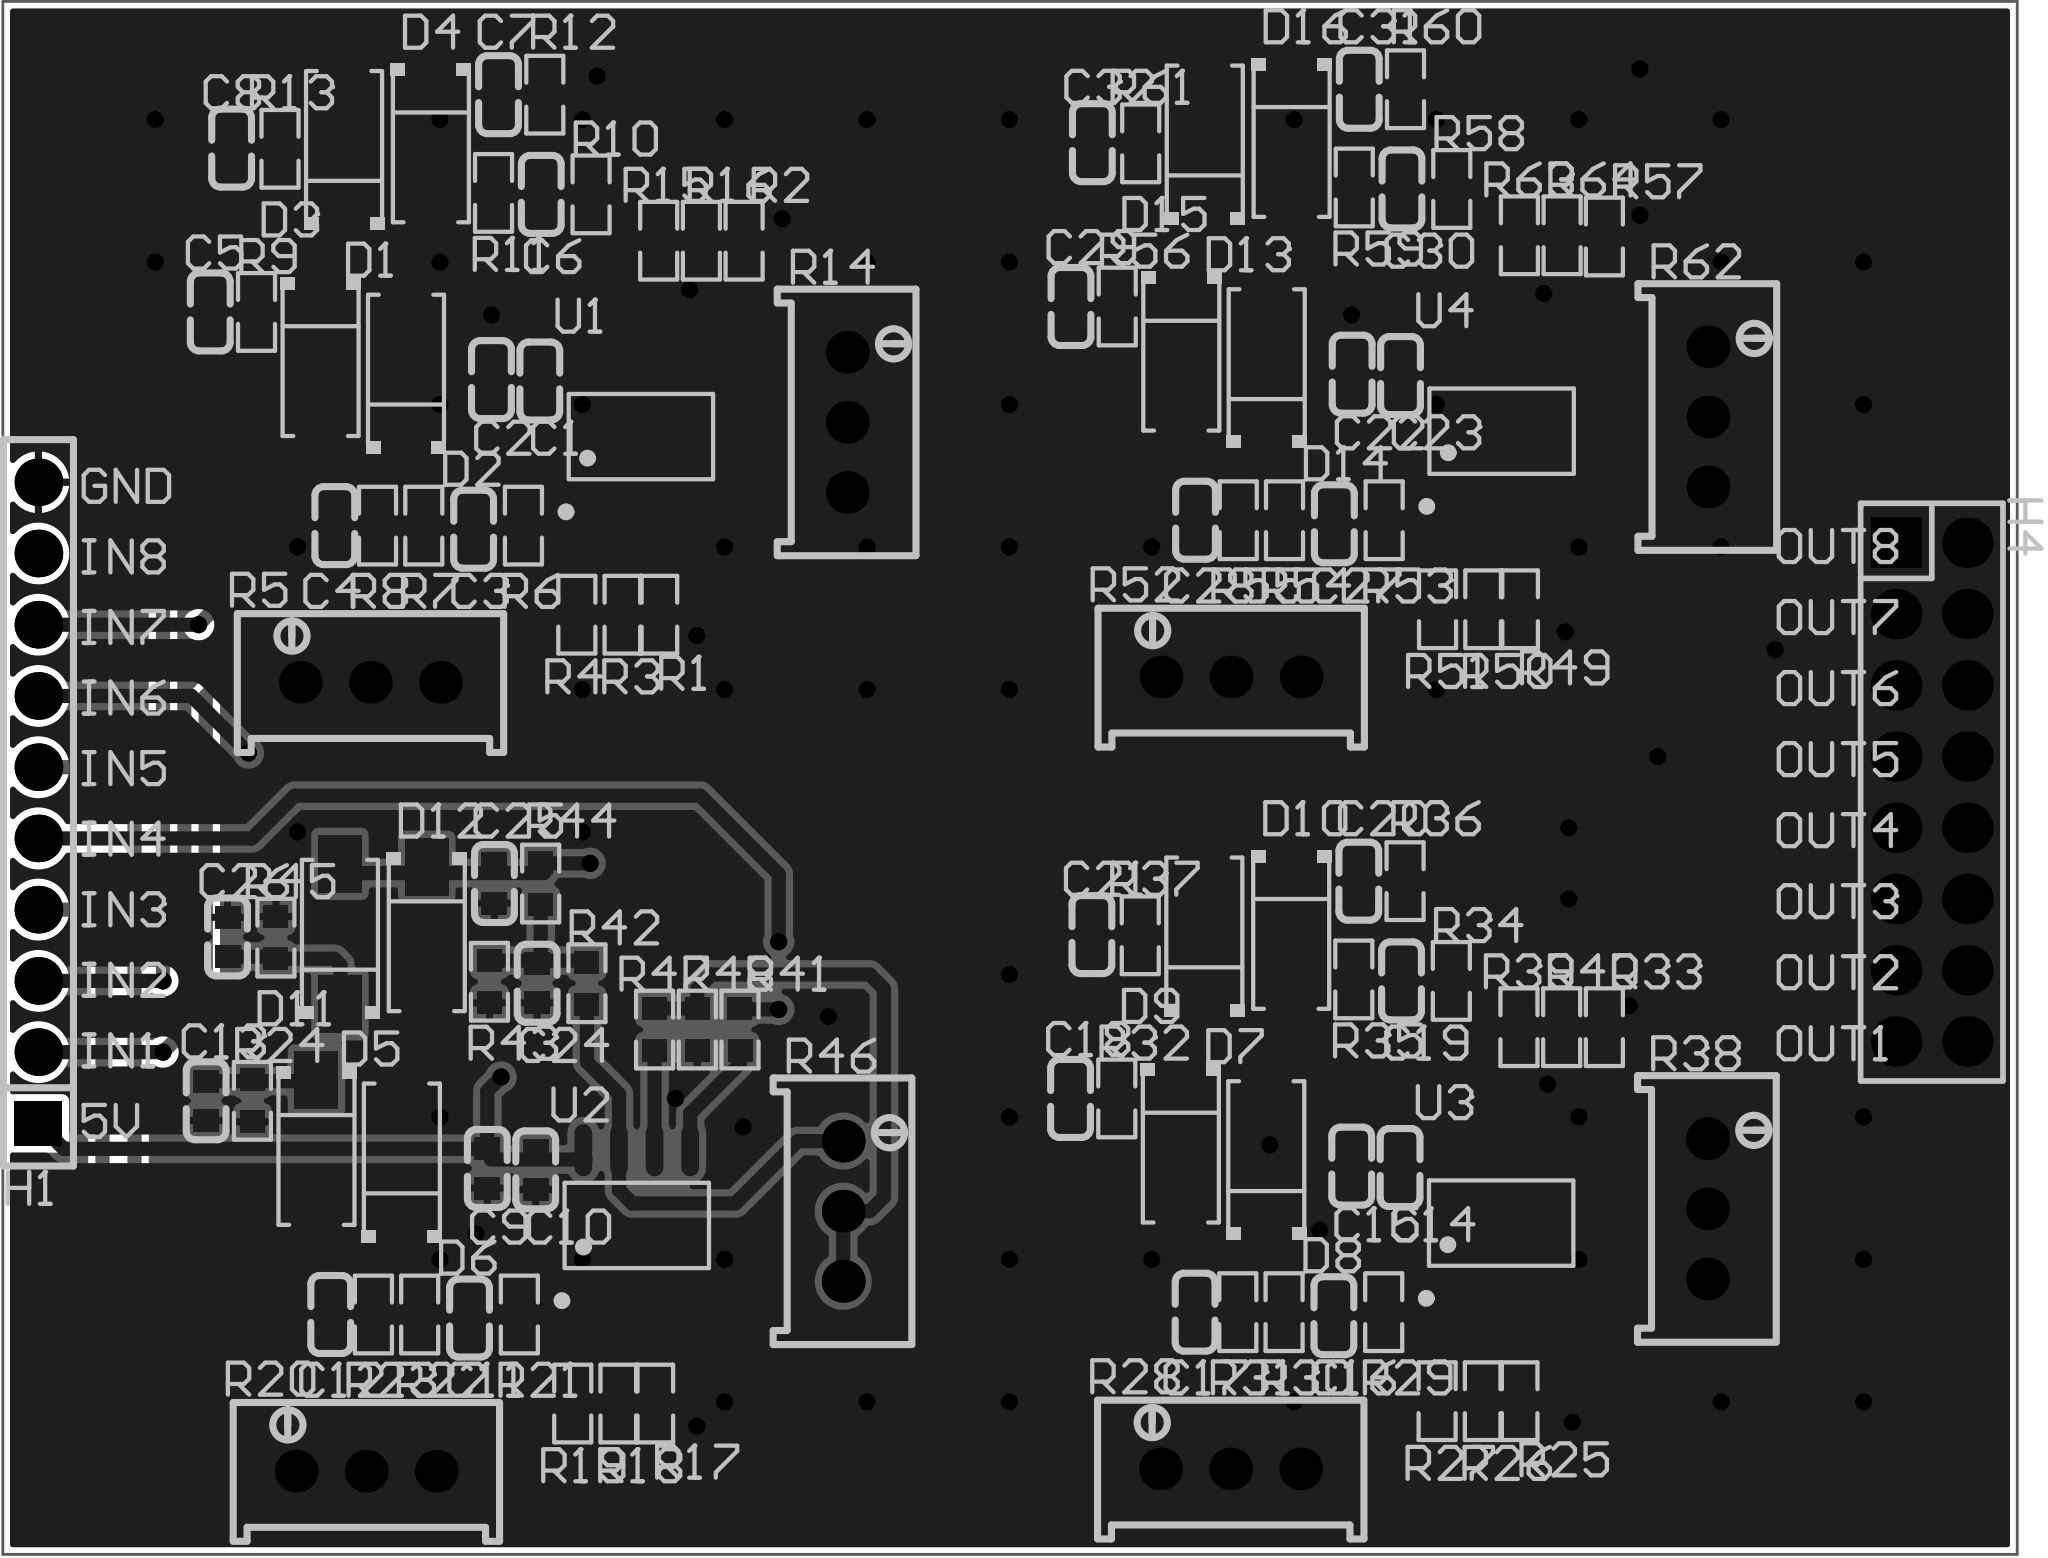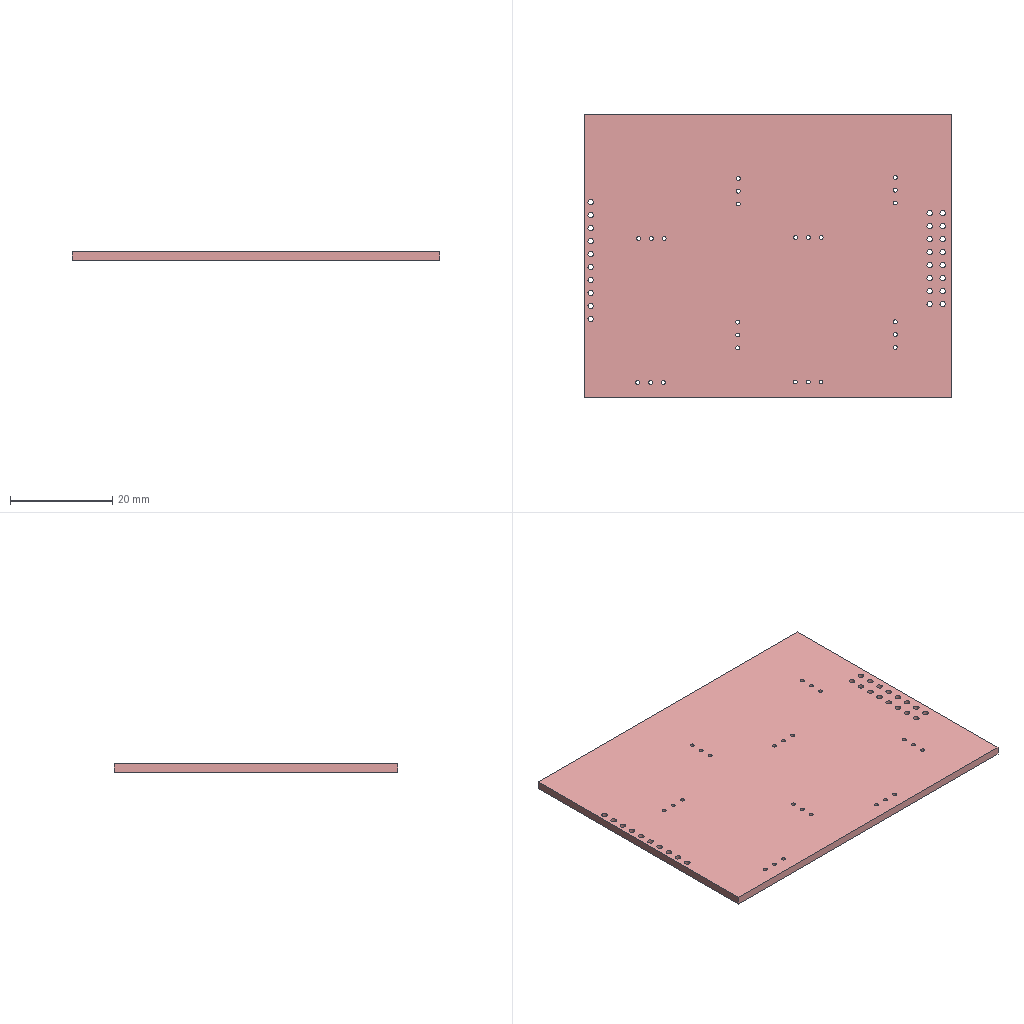Circuit board layout | Altium Designer | box 71.9 x 55.4 x 1.6 mm
Layer stack:
# Altium Designer layer stack of  (unit mm; dielectric type: 0 none, 1 core, 2 prepreg, 3 surface material)
index,name,kind,layer,copper_thickness_mm,dielectric_type,dielectric_thickness_mm,dielectric_material,dielectric_constant
0,Top Paste Mask Layer,other,,,,,,
1,Top Silkscreen Layer,other,,,,,,
2,Top Solder Mask Layer,dielectric,,,3,0.01,,3.3
3,Top Layer,copper,Top Layer,0.035,,,,
4,Dielectric1,dielectric,,,3,1.51,FR4,4.5
5,Bottom Layer,copper,Bottom Layer,0.035,,,,
6,Bottom Solder Mask Layer,dielectric,,,3,0.01,,3.3
7,Bottom Silkscreen Layer,other,,,,,,
8,Bottom Paste Mask Layer,other,,,,,,
# drill layer pairs: low layer,high layer
drill_pair,Top Layer,Bottom Layer
Part placement:
Designator,Comment,Layer,Footprint,Center-X(mm),Center-Y(mm),Rotation
C1,100nF,TopLayer,C0603,106.791,128.197,90
C2,10uF,TopLayer,C0603,105.065,128.247,90
C3,10uF,TopLayer,C0603,104.43,122.913,270
C4,100nF,TopLayer,C0603,99.477,123.04,90
C5,100nF,TopLayer,C0603,95.032,130.66,90
C6,10uF,TopLayer,C0603,106.843,134.851,90
C7,100nF,TopLayer,C0603,105.319,138.407,90
C8,100nF,TopLayer,C0603,95.794,136.502,270
C9,100nF,TopLayer,C0603,104.918,100.12,90
C10,10uF,TopLayer,C0603,106.645,100.069,90
C11,10uF,TopLayer,C0603,104.283,94.786,270
C12,100nF,TopLayer,C0603,99.33,94.913,90
C13,100nF,TopLayer,C0603,94.885,102.533,90
C14,100nF,TopLayer,C0603,137.49,100.153,90
C15,10uF,TopLayer,C0603,135.763,100.203,90
C16,10uF,TopLayer,C0603,135.128,94.869,270
C17,100nF,TopLayer,C0603,130.175,94.996,90
C18,100nF,TopLayer,C0603,125.73,102.616,90
C19,10uF,TopLayer,C0603,137.541,106.807,90
C20,100nF,TopLayer,C0603,136.017,110.363,90
C21,100nF,TopLayer,C0603,126.492,108.458,270
C22,100nF,TopLayer,C0603,135.779,128.441,90
C23,10uF,TopLayer,C0603,137.506,128.39,90
C24,10uF,TopLayer,C0603,106.696,106.724,90
C25,100nF,TopLayer,C0603,105.172,110.28,90
C26,100nF,TopLayer,C0603,95.647,108.375,270
C27,10uF,TopLayer,C0603,135.144,123.107,270
C28,100nF,TopLayer,C0603,130.191,123.234,90
C29,100nF,TopLayer,C0603,125.746,130.854,90
C30,10uF,TopLayer,C0603,137.557,135.044,90
C31,100nF,TopLayer,C0603,136.033,138.601,90
C32,100nF,TopLayer,C0603,126.508,136.696,270
D1,SS54,TopLayer,SMA_L4.4-W2.8-LS5.4-R-RD,98.969,128.882,270
D2,SS54,TopLayer,SMA_L4.4-W2.8-LS5.4-R-RD,102.017,128.628,90
D3,SS54,TopLayer,SMA_L4.4-W2.8-LS5.4-R-RD,99.806,136.604,90
D4,SS54,TopLayer,SMA_L4.4-W2.8-LS5.4-R-RD,102.906,136.502,270
D5,SS54,TopLayer,SMA_L4.4-W2.8-LS5.4-R-RD,98.822,100.755,270
D6,SS54,TopLayer,SMA_L4.4-W2.8-LS5.4-R-RD,101.87,100.501,90
D7,SS54,TopLayer,SMA_L4.4-W2.8-LS5.4-R-RD,129.667,100.838,270
D8,SS54,TopLayer,SMA_L4.4-W2.8-LS5.4-R-RD,132.715,100.584,90
D9,SS54,TopLayer,SMA_L4.4-W2.8-LS5.4-R-RD,130.505,108.56,90
D10,SS54,TopLayer,SMA_L4.4-W2.8-LS5.4-R-RD,133.604,108.458,270
D11,SS54,TopLayer,SMA_L4.4-W2.8-LS5.4-R-RD,99.66,108.477,90
D12,SS54,TopLayer,SMA_L4.4-W2.8-LS5.4-R-RD,102.759,108.375,270
D13,SS54,TopLayer,SMA_L4.4-W2.8-LS5.4-R-RD,129.683,129.076,270
D14,SS54,TopLayer,SMA_L4.4-W2.8-LS5.4-R-RD,132.731,128.822,90
D15,SS54,TopLayer,SMA_L4.4-W2.8-LS5.4-R-RD,130.521,136.798,90
D16,SS54,TopLayer,SMA_L4.4-W2.8-LS5.4-R-RD,133.62,136.696,270
H1,,TopLayer,HDR-TH_10P-P2.54-V-F,88.9,113.157,90
H4,,TopLayer,HDR-TH_16P-P2.54-V-F-R2-C8-S2.54-1,156.464,113.538,270
R1,10K,TopLayer,R0603,111.034,119.865,90
R2,10K,TopLayer,R0603,114.082,133.2,270
R3,10K,TopLayer,R0603,109.764,119.865,90
R4,1K,TopLayer,R0603,108.113,119.865,270
R5,10kΩ,TopLayer,RES-ADJ-TH_3P-L10.0-W10.0-P2.50-L,100.747,117.452,0
R6,1K,TopLayer,R0603,106.208,123.04,90
R7,10K,TopLayer,R0603,102.652,123.04,270
R8,1K,TopLayer,R0603,101.001,123.04,90
R9,10K,TopLayer,R0603,96.683,130.66,270
R10,1K,TopLayer,R0603,108.621,134.851,270
R11,10K,TopLayer,R0603,105.14,134.904,90
R12,1K,TopLayer,R0603,106.97,138.407,90
R13,10K,TopLayer,R0603,97.52,136.477,90
R14,10kΩ,TopLayer,RES-ADJ-TH_3P-L10.0-W10.0-P2.50-L,117.765,126.723,270
R15,10K,TopLayer,R0603,111.034,133.2,270
R16,1K,TopLayer,R0603,112.558,133.2,90
R17,10K,TopLayer,R0603,110.887,91.738,90
R18,10K,TopLayer,R0603,109.617,91.738,90
R19,1K,TopLayer,R0603,107.966,91.738,270
R20,10kΩ,TopLayer,RES-ADJ-TH_3P-L10.0-W10.0-P2.50-L,100.6,89.325,0
R21,1K,TopLayer,R0603,106.061,94.913,90
R22,10K,TopLayer,R0603,102.505,94.913,270
R23,1K,TopLayer,R0603,100.854,94.913,90
R24,10K,TopLayer,R0603,96.536,102.533,270
R25,10K,TopLayer,R0603,141.732,91.821,90
R26,10K,TopLayer,R0603,140.462,91.821,90
R27,1K,TopLayer,R0603,138.811,91.821,270
R28,10kΩ,TopLayer,RES-ADJ-TH_3P-L10.0-W10.0-P2.50-L,131.445,89.408,0
R29,1K,TopLayer,R0603,136.906,94.996,90
R30,10K,TopLayer,R0603,133.35,94.996,270
R31,1K,TopLayer,R0603,131.699,94.996,90
R32,10K,TopLayer,R0603,127.381,102.616,270
R33,10K,TopLayer,R0603,144.78,105.156,270
R34,1K,TopLayer,R0603,139.319,106.807,270
R35,10K,TopLayer,R0603,135.839,106.86,90
R36,1K,TopLayer,R0603,137.668,110.363,90
R37,10K,TopLayer,R0603,128.219,108.433,90
R38,10kΩ,TopLayer,RES-ADJ-TH_3P-L10.0-W10.0-P2.50-L,148.463,98.679,270
R39,10K,TopLayer,R0603,141.732,105.156,270
R40,1K,TopLayer,R0603,143.256,105.156,90
R41,10K,TopLayer,R0603,113.935,105.073,270
R42,1K,TopLayer,R0603,108.474,106.724,270
R43,10K,TopLayer,R0603,104.994,106.776,90
R44,1K,TopLayer,R0603,106.823,110.28,90
R45,10K,TopLayer,R0603,97.374,108.35,90
R46,10kΩ,TopLayer,RES-ADJ-TH_3P-L10.0-W10.0-P2.50-L,117.618,98.596,270
R47,10K,TopLayer,R0603,110.887,105.073,270
R48,1K,TopLayer,R0603,112.411,105.073,90
R49,10K,TopLayer,R0603,141.748,120.059,90
R50,10K,TopLayer,R0603,140.478,120.059,90
R51,1K,TopLayer,R0603,138.827,120.059,270
R52,10kΩ,TopLayer,RES-ADJ-TH_3P-L10.0-W10.0-P2.50-L,131.461,117.646,0
R53,1K,TopLayer,R0603,136.922,123.234,90
R54,10K,TopLayer,R0603,133.366,123.234,270
R55,1K,TopLayer,R0603,131.715,123.234,90
R56,10K,TopLayer,R0603,127.397,130.854,270
R57,10K,TopLayer,R0603,144.78,133.35,270
R58,1K,TopLayer,R0603,139.335,135.044,270
R59,10K,TopLayer,R0603,135.855,135.097,90
R60,1K,TopLayer,R0603,137.684,138.601,90
R61,10K,TopLayer,R0603,128.235,136.671,90
R62,10kΩ,TopLayer,RES-ADJ-TH_3P-L10.0-W10.0-P2.50-L,148.479,126.917,270
R63,10K,TopLayer,R0603,141.748,133.394,270
R64,1K,TopLayer,R0603,143.272,133.394,90
U1,LM358DR-CN,TopLayer,SOIC-8_L4.9-W4.0-P1.27-LS6.0-BL,110.399,126.215,0
U2,LM358DR-CN,TopLayer,SOIC-8_L4.9-W4.0-P1.27-LS6.0-BL,110.252,98.088,0
U3,LM358DR-CN,TopLayer,SOIC-8_L4.9-W4.0-P1.27-LS6.0-BL,141.097,98.171,0
U4,LM358DR-CN,TopLayer,SOIC-8_L4.9-W4.0-P1.27-LS6.0-BL,141.113,126.409,0
Pad and via stacks:
# Altium Designer via and pad stacks of  (unit mm). Each distinct definition once, with the count of objects using it.
# via: kind,start_layer,end_layer,hole_mm,diameter_mm,mode(0 simple;1 top-mid-bottom;2 full stack),diameter_per_layer,count,example_net
# pad: kind,layer,hole_mm,hole_type(0 round;1 square;2 slot),plating,top_size,top_shape(1 round;2 rect;3 octagon;9 rounded rect),mid_size,bottom_size,mode,footprint,size_per_layer,count,example
pad,Top Layer,0,0,plated,0.8x0.9,2,0.8x0.9,0.8x0.9,0,C0603,,64,C1.2
pad,Top Layer,0,0,plated,2.062x1.539,2,2.062x1.539,2.062x1.539,0,SMA_L4.4-W2.8-LS5.4-R-RD,,32,D1.1
pad,Top Layer,0,0,plated,0.8065x0.864,2,0.8065x0.864,0.8065x0.864,0,R0603,,112,R1.2
pad,Top Layer,0,0,plated,0.63x1.865,1,0.63x1.865,0.63x1.865,0,SOIC-8_L4.9-W4.0-P1.27-LS6.0-BL,,32,U1.1
pad,Multi-Layer,1.1,0,plated,1.7x1.7,1,1.7x1.7,1.7x1.7,0,HDR-TH_10P-P2.54-V-F,,9,H1.10
pad,Multi-Layer,1.1,0,plated,1.575x1.7,2,1.575x1.7,1.575x1.7,0,HDR-TH_10P-P2.54-V-F,,1,H1.1
pad,Multi-Layer,1.1,0,plated,1.8x1.8,1,1.8x1.8,1.8x1.8,0,HDR-TH_16P-P2.54-V-F-R2-C8-S2.54-1,,15,H4.16
pad,Multi-Layer,1.1,0,plated,1.8x1.8,2,1.8x1.8,1.8x1.8,0,HDR-TH_16P-P2.54-V-F-R2-C8-S2.54-1,,1,H4.1
pad,Multi-Layer,0.762,0,plated,1.524x1.524,1,1.524x1.524,1.524x1.524,0,RES-ADJ-TH_3P-L10.0-W10.0-P2.50-L,,24,R5.2
via,Top Layer,Bottom Layer,0.3048,0.61,0,,85,OUT8
Copper pours:
name,layer,net,type(0 solid;1 hatched;2 none)
Top Layer-GND,Top Layer,GND,0
Bottom Layer-GND,Bottom Layer,GND,0
Design rules, without the lines most boards share:
# Altium Designer design rules of  (exported by Altium Designer, unit mm)
# columns: name | kind | enabled | priority | scope1 | scope2 | descriptor | typed fields (field=value)
creepage | 65 | enabled | 1 | All | All | Creepage Distance Constraint =(0mil) (All),(All) |